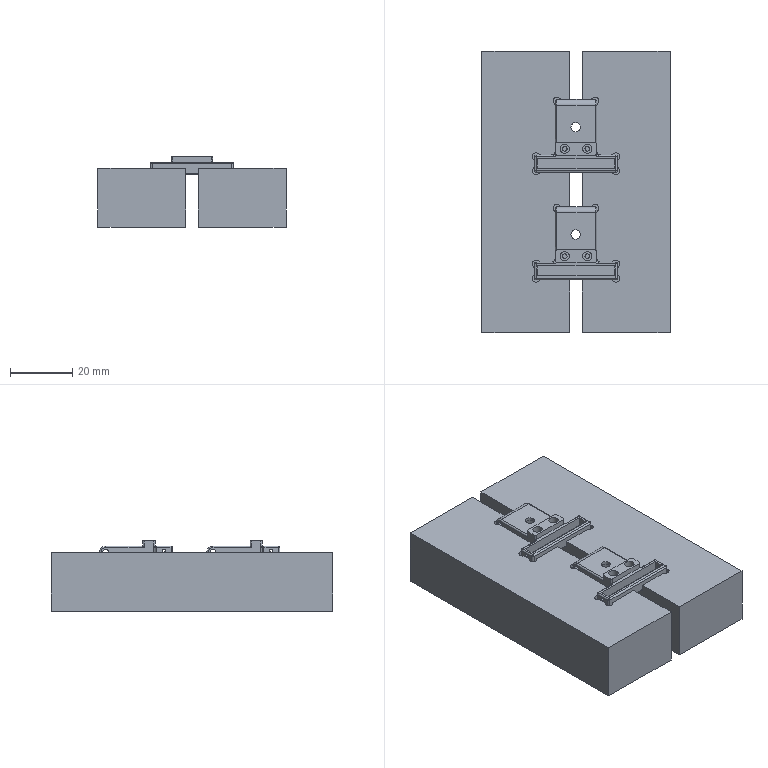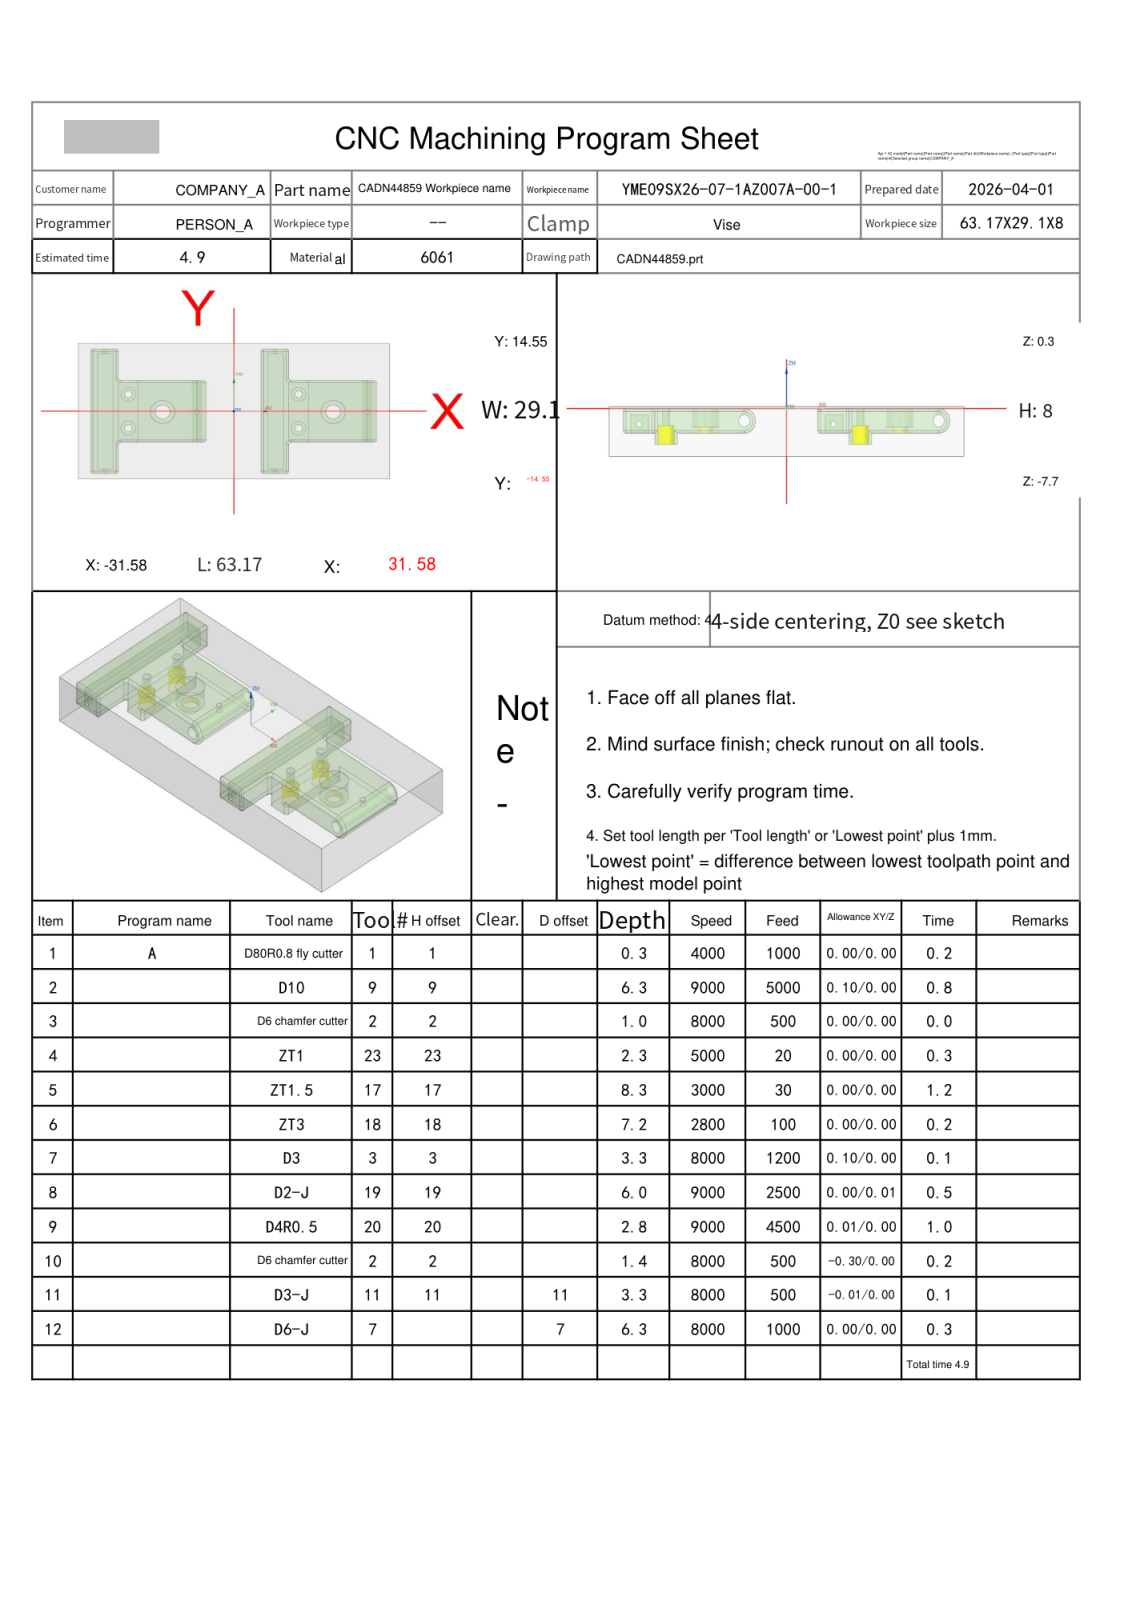NC program | NX | posted by the shop | part box 60.696 x 90.669 x 22.754 mm
Lines 1 to 833 of 3978:
%
O0001
(Machine time: 7.16 MIN)
(===Total Tool:11===)
(T1=D80R0.8 fly cutter D=80.  R=0.8  D-  H01 Z=0.    )
(T9=D10     D=10.  R=0.   D-  H09 Z=-5.95 )
(T2=D6 chamfer cutter   D=6.   R=0.   D-  H02 Z=-1.05 )
(T23=ZT1    D=1.   DR_a=118 D-  H23 Z=-2.   )
(T17=ZT1.5  D=1.5  DR_a=118 D-  H17 Z=-8.   )
(T18=ZT3    D=3.   DR_a=118 D-  H18 Z=-6.9  )
(T3=D3      D=3.   R=0.   D-  H03 Z=-3.   )
(T19=D2-J   D=2.   R=0.   D-  H19 Z=-5.7  )
(T20=D4R0.5 D=4.   R=0.5  D-  H20 Z=-2.5  )
(T11=D3-J   D=3.   R=0.   D11 H11 Z=-3.   )
(T7=D6-J    D=6.   R=0.   D7  H00 Z=-5.95 )
G80 G90 G17 G49 G40
G91 G28 Z0
M01
N1 T01 M06
(D80R0.8 fly cutter  D=80. R=0.8 H=01 ce=0.00 di=0.00)
G00 G90 G54 X-74.084 Y0.0 M03 S4000
G43 H01 Z20.
M08
Z2.
G01 Z0.0 F1000.
X-69.084
X69.084
X74.084
Z2.
G00 Z20.
G91 G28 Z0.0
M05
M09
G91 G28 Z0.0
M01
N2 T09 M06
(D10  D=10. R=0. H=09 ce=0.10 di=0.00)
G00 G90 G54 X.416 Y0.0 M03 S8000
G43 H09 Z20.
M08
Z.5
G01 Y12.848 Z.427 F5000.
G02 X6.016 Y18.448 Z.378 I5.6 J0.0
G01 X10.648 Z.352
G02 X16.248 Y12.848 Z.302 I0.0 J-5.6
G01 Y11.734 Z.296
X28.584 Z.226
G02 X34.184 Y6.134 Z.176 I0.0 J-5.6
G01 Y-6.134 Z.107
G02 X28.584 Y-11.734 Z.057 I-5.6 J0.0
G01 X16.248 Z-.013
Y-12.848 Z-.019
G02 X10.648 Y-18.448 Z-.069 I-5.6 J0.0
G01 X6.016 Z-.095
G02 X.416 Y-12.848 Z-.145 I0.0 J5.6
G01 Y12.848 Z-.29
G02 X6.016 Y18.448 Z-.339 I5.6 J0.0
G01 X10.648 Z-.366
G02 X16.248 Y12.848 Z-.415 I0.0 J-5.6
G01 Y11.734 Z-.422
X28.584 Z-.491
G02 X34.184 Y6.134 Z-.541 I0.0 J-5.6
G01 Y-6.134 Z-.61
G02 X28.584 Y-11.734 Z-.66 I-5.6 J0.0
G01 X16.248 Z-.73
Y-12.848 Z-.736
G02 X10.648 Y-18.448 Z-.786 I-5.6 J0.0
G01 X6.016 Z-.812
G02 X.416 Y-12.848 Z-.862 I0.0 J5.6
G01 Y12.848 Z-1.007
G02 X6.016 Y18.448 Z-1.057 I5.6 J0.0
G01 X10.648 Z-1.083
G02 X16.248 Y12.848 Z-1.132 I0.0 J-5.6
G01 Y11.734 Z-1.139
X28.584 Z-1.208
G02 X34.184 Y6.134 Z-1.258 I0.0 J-5.6
G01 Y-6.134 Z-1.327
G02 X28.584 Y-11.734 Z-1.377 I-5.6 J0.0
G01 X16.248 Z-1.447
Y-12.848 Z-1.453
G02 X10.648 Y-18.448 Z-1.503 I-5.6 J0.0
G01 X6.016 Z-1.529
G02 X.416 Y-12.848 Z-1.579 I0.0 J5.6
G01 Y12.848 Z-1.724
G02 X6.016 Y18.448 Z-1.774 I5.6 J0.0
G01 X10.648 Z-1.8
G02 X16.248 Y12.848 Z-1.85 I0.0 J-5.6
G01 Y11.734 Z-1.856
X28.584 Z-1.926
G02 X34.184 Y6.134 Z-1.975 I0.0 J-5.6
G01 Y-6.134 Z-2.045
G02 X28.584 Y-11.734 Z-2.094 I-5.6 J0.0
G01 X16.248 Z-2.164
Y-12.848 Z-2.17
G02 X10.648 Y-18.448 Z-2.22 I-5.6 J0.0
G01 X6.016 Z-2.246
G02 X.416 Y-12.848 Z-2.296 I0.0 J5.6
G01 Y12.848 Z-2.441
G02 X6.016 Y18.448 Z-2.491 I5.6 J0.0
G01 X10.648 Z-2.517
G02 X16.248 Y12.848 Z-2.567 I0.0 J-5.6
G01 Y11.734 Z-2.573
X28.584 Z-2.643
G02 X34.184 Y6.134 Z-2.692 I0.0 J-5.6
G01 Y-6.134 Z-2.762
G02 X28.584 Y-11.734 Z-2.811 I-5.6 J0.0
G01 X16.248 Z-2.881
Y-12.848 Z-2.887
G02 X10.648 Y-18.448 Z-2.937 I-5.6 J0.0
G01 X6.016 Z-2.963
G02 X.416 Y-12.848 Z-3.013 I0.0 J5.6
G01 Y12.848 Z-3.158
G02 X6.016 Y18.448 Z-3.208 I5.6 J0.0
G01 X10.648 Z-3.234
G02 X16.248 Y12.848 Z-3.284 I0.0 J-5.6
G01 Y11.734 Z-3.29
X28.584 Z-3.36
G02 X34.184 Y6.134 Z-3.409 I0.0 J-5.6
G01 Y-6.134 Z-3.479
G02 X28.584 Y-11.734 Z-3.528 I-5.6 J0.0
G01 X16.248 Z-3.598
Y-12.848 Z-3.605
G02 X10.648 Y-18.448 Z-3.654 I-5.6 J0.0
G01 X6.016 Z-3.68
G02 X.416 Y-12.848 Z-3.73 I0.0 J5.6
G01 Y12.848 Z-3.875
G02 X6.016 Y18.448 Z-3.925 I5.6 J0.0
G01 X10.648 Z-3.951
G02 X16.248 Y12.848 Z-4.001 I0.0 J-5.6
G01 Y11.734 Z-4.007
X28.584 Z-4.077
G02 X34.184 Y6.134 Z-4.127 I0.0 J-5.6
G01 Y-6.134 Z-4.196
G02 X28.584 Y-11.734 Z-4.246 I-5.6 J0.0
G01 X16.248 Z-4.315
Y-12.848 Z-4.322
G02 X10.648 Y-18.448 Z-4.371 I-5.6 J0.0
G01 X6.016 Z-4.397
G02 X.416 Y-12.848 Z-4.447 I0.0 J5.6
G01 Y12.848 Z-4.592
G02 X6.016 Y18.448 Z-4.642 I5.6 J0.0
G01 X10.648 Z-4.668
G02 X16.248 Y12.848 Z-4.718 I0.0 J-5.6
G01 Y11.734 Z-4.724
X28.584 Z-4.794
G02 X34.184 Y6.134 Z-4.844 I0.0 J-5.6
G01 Y-6.134 Z-4.913
G02 X28.584 Y-11.734 Z-4.963 I-5.6 J0.0
G01 X16.248 Z-5.032
Y-12.848 Z-5.039
G02 X10.648 Y-18.448 Z-5.088 I-5.6 J0.0
G01 X6.016 Z-5.115
G02 X.416 Y-12.848 Z-5.164 I0.0 J5.6
G01 Y12.848 Z-5.31
G02 X6.016 Y18.448 Z-5.359 I5.6 J0.0
G01 X10.648 Z-5.385
G02 X16.248 Y12.848 Z-5.435 I0.0 J-5.6
G01 Y11.734 Z-5.441
X28.584 Z-5.511
G02 X34.184 Y6.134 Z-5.561 I0.0 J-5.6
G01 Y-6.134 Z-5.63
G02 X28.584 Y-11.734 Z-5.68 I-5.6 J0.0
G01 X16.248 Z-5.75
Y-12.848 Z-5.756
G02 X10.648 Y-18.448 Z-5.806 I-5.6 J0.0
G01 X6.016 Z-5.832
G02 X.416 Y-12.848 Z-5.881 I0.0 J5.6
G01 Y0.0 Z-5.954
Y12.848
G02 X6.016 Y18.448 I5.6 J0.0
G01 X10.648
G02 X16.248 Y12.848 I0.0 J-5.6
G01 Y11.734
X28.584
G02 X34.184 Y6.134 I0.0 J-5.6
G01 Y-6.134
G02 X28.584 Y-11.734 I-5.6 J0.0
G01 X16.248
Y-12.848
G02 X10.648 Y-18.448 I-5.6 J0.0
G01 X6.016
G02 X.416 Y-12.848 I0.0 J5.6
G01 Y0.0
Y.5
Z-4.954
G00 Z20.
X-34.184 Y0.0
Z.5
G01 Y12.848 Z.427
G02 X-28.584 Y18.448 Z.378 I5.6 J0.0
G01 X-23.952 Z.352
G02 X-18.352 Y12.848 Z.302 I0.0 J-5.6
G01 Y11.734 Z.296
X-6.016 Z.226
G02 X-.416 Y6.134 Z.176 I0.0 J-5.6
G01 Y-6.134 Z.107
G02 X-6.016 Y-11.734 Z.057 I-5.6 J0.0
G01 X-18.352 Z-.013
Y-12.848 Z-.019
G02 X-23.952 Y-18.448 Z-.069 I-5.6 J0.0
G01 X-28.584 Z-.095
G02 X-34.184 Y-12.848 Z-.145 I0.0 J5.6
G01 Y12.848 Z-.29
G02 X-28.584 Y18.448 Z-.339 I5.6 J0.0
G01 X-23.952 Z-.366
G02 X-18.352 Y12.848 Z-.415 I0.0 J-5.6
G01 Y11.734 Z-.422
X-6.016 Z-.491
G02 X-.416 Y6.134 Z-.541 I0.0 J-5.6
G01 Y-6.134 Z-.61
G02 X-6.016 Y-11.734 Z-.66 I-5.6 J0.0
G01 X-18.352 Z-.73
Y-12.848 Z-.736
G02 X-23.952 Y-18.448 Z-.786 I-5.6 J0.0
G01 X-28.584 Z-.812
G02 X-34.184 Y-12.848 Z-.862 I0.0 J5.6
G01 Y12.848 Z-1.007
G02 X-28.584 Y18.448 Z-1.057 I5.6 J0.0
G01 X-23.952 Z-1.083
G02 X-18.352 Y12.848 Z-1.132 I0.0 J-5.6
G01 Y11.734 Z-1.139
X-6.016 Z-1.208
G02 X-.416 Y6.134 Z-1.258 I0.0 J-5.6
G01 Y-6.134 Z-1.327
G02 X-6.016 Y-11.734 Z-1.377 I-5.6 J0.0
G01 X-18.352 Z-1.447
Y-12.848 Z-1.453
G02 X-23.952 Y-18.448 Z-1.503 I-5.6 J0.0
G01 X-28.584 Z-1.529
G02 X-34.184 Y-12.848 Z-1.579 I0.0 J5.6
G01 Y12.848 Z-1.724
G02 X-28.584 Y18.448 Z-1.774 I5.6 J0.0
G01 X-23.952 Z-1.8
G02 X-18.352 Y12.848 Z-1.85 I0.0 J-5.6
G01 Y11.734 Z-1.856
X-6.016 Z-1.926
G02 X-.416 Y6.134 Z-1.975 I0.0 J-5.6
G01 Y-6.134 Z-2.045
G02 X-6.016 Y-11.734 Z-2.094 I-5.6 J0.0
G01 X-18.352 Z-2.164
Y-12.848 Z-2.17
G02 X-23.952 Y-18.448 Z-2.22 I-5.6 J0.0
G01 X-28.584 Z-2.246
G02 X-34.184 Y-12.848 Z-2.296 I0.0 J5.6
G01 Y12.848 Z-2.441
G02 X-28.584 Y18.448 Z-2.491 I5.6 J0.0
G01 X-23.952 Z-2.517
G02 X-18.352 Y12.848 Z-2.567 I0.0 J-5.6
G01 Y11.734 Z-2.573
X-6.016 Z-2.643
G02 X-.416 Y6.134 Z-2.692 I0.0 J-5.6
G01 Y-6.134 Z-2.762
G02 X-6.016 Y-11.734 Z-2.811 I-5.6 J0.0
G01 X-18.352 Z-2.881
Y-12.848 Z-2.887
G02 X-23.952 Y-18.448 Z-2.937 I-5.6 J0.0
G01 X-28.584 Z-2.963
G02 X-34.184 Y-12.848 Z-3.013 I0.0 J5.6
G01 Y12.848 Z-3.158
G02 X-28.584 Y18.448 Z-3.208 I5.6 J0.0
G01 X-23.952 Z-3.234
G02 X-18.352 Y12.848 Z-3.284 I0.0 J-5.6
G01 Y11.734 Z-3.29
X-6.016 Z-3.36
G02 X-.416 Y6.134 Z-3.409 I0.0 J-5.6
G01 Y-6.134 Z-3.479
G02 X-6.016 Y-11.734 Z-3.528 I-5.6 J0.0
G01 X-18.352 Z-3.598
Y-12.848 Z-3.605
G02 X-23.952 Y-18.448 Z-3.654 I-5.6 J0.0
G01 X-28.584 Z-3.68
G02 X-34.184 Y-12.848 Z-3.73 I0.0 J5.6
G01 Y12.848 Z-3.875
G02 X-28.584 Y18.448 Z-3.925 I5.6 J0.0
G01 X-23.952 Z-3.951
G02 X-18.352 Y12.848 Z-4.001 I0.0 J-5.6
G01 Y11.734 Z-4.007
X-6.016 Z-4.077
G02 X-.416 Y6.134 Z-4.127 I0.0 J-5.6
G01 Y-6.134 Z-4.196
G02 X-6.016 Y-11.734 Z-4.246 I-5.6 J0.0
G01 X-18.352 Z-4.315
Y-12.848 Z-4.322
G02 X-23.952 Y-18.448 Z-4.371 I-5.6 J0.0
G01 X-28.584 Z-4.397
G02 X-34.184 Y-12.848 Z-4.447 I0.0 J5.6
G01 Y12.848 Z-4.592
G02 X-28.584 Y18.448 Z-4.642 I5.6 J0.0
G01 X-23.952 Z-4.668
G02 X-18.352 Y12.848 Z-4.718 I0.0 J-5.6
G01 Y11.734 Z-4.724
X-6.016 Z-4.794
G02 X-.416 Y6.134 Z-4.844 I0.0 J-5.6
G01 Y-6.134 Z-4.913
G02 X-6.016 Y-11.734 Z-4.963 I-5.6 J0.0
G01 X-18.352 Z-5.032
Y-12.848 Z-5.039
G02 X-23.952 Y-18.448 Z-5.088 I-5.6 J0.0
G01 X-28.584 Z-5.115
G02 X-34.184 Y-12.848 Z-5.164 I0.0 J5.6
G01 Y12.848 Z-5.31
G02 X-28.584 Y18.448 Z-5.359 I5.6 J0.0
G01 X-23.952 Z-5.385
G02 X-18.352 Y12.848 Z-5.435 I0.0 J-5.6
G01 Y11.734 Z-5.441
X-6.016 Z-5.511
G02 X-.416 Y6.134 Z-5.561 I0.0 J-5.6
G01 Y-6.134 Z-5.63
G02 X-6.016 Y-11.734 Z-5.68 I-5.6 J0.0
G01 X-18.352 Z-5.75
Y-12.848 Z-5.756
G02 X-23.952 Y-18.448 Z-5.806 I-5.6 J0.0
G01 X-28.584 Z-5.832
G02 X-34.184 Y-12.848 Z-5.881 I0.0 J5.6
G01 Y0.0 Z-5.954
Y12.848
G02 X-28.584 Y18.448 I5.6 J0.0
G01 X-23.952
G02 X-18.352 Y12.848 I0.0 J-5.6
G01 Y11.734
X-6.016
G02 X-.416 Y6.134 I0.0 J-5.6
G01 Y-6.134
G02 X-6.016 Y-11.734 I-5.6 J0.0
G01 X-18.352
Y-12.848
G02 X-23.952 Y-18.448 I-5.6 J0.0
G01 X-28.584
G02 X-34.184 Y-12.848 I0.0 J5.6
G01 Y0.0
Y.5
Z-4.954
G00 Z20.
G00 G90 X-13.625 Y16.359 M03 S9000
Z10.3
Z.484
G01 Z-.016 F4500.
G03 X-8.625 Y11.359 I5. J0.0
G02 X-7.98 Y11.389 I.645 J-7.027
X-5.459 Y10.923 I0.0 J-7.056
X-2.164 Y6.134 I-1.832 J-4.788
G01 Y-6.134
G02 X-7.305 Y-11.341 I-5.311 J.102
G01 X-8.625 Y-11.359
X-8.627 Y-11.406 Z-.031
X-8.629 Y-11.438 Z-.045
X-7.544
X-7.305 Y-11.43
G03 X-2. Y-6.134 I-.154 J5.46
G01 Y6.134
G03 X-6.404 Y11.319 I-5.4 J-.123
X-8.1 Y11.451 I-1.696 J-10.865
X-8.629 Y11.438 I0.0 J-10.996
G01 Y11.489 Z-.07
Y11.525 Z-.095
G02 X-8.055 Y11.539 I.574 J-11.406
X-6.349 Y11.411 I0.0 J-11.42
X-1.812 Y6.134 I-.964 J-5.417
G01 Y-6.134
G02 X-5.053 Y-11.009 I-5.387 J.067
X-7.498 Y-11.521 I-2.445 J5.587
G01 X-7.544
X-8.614
X-8.629 Y-11.525
Y-11.606 Z-.166
X-8.614 Y-11.601
X-7.468 Y-11.6
G03 X-4.683 Y-10.963 I-.002 J6.41
X-1.618 Y-6.134 I-2.358 J4.883
G01 Y6.134
G03 X-2.579 Y9.173 I-5.492 J-.064
X-7.017 Y11.582 I-4.734 J-3.43
X-8.148 Y11.611 I-1.132 J-22.252
X-8.629 Y11.606 I0.0 J-22.281
G01 X-8.628 Y11.641 Z-.209
Y11.669 Z-.253
G02 X-8.102 Y11.675 I.526 J-20.023
X-6.855 Y11.637 I0.0 J-20.03
X-4.152 Y10.804 I-.457 J-6.288
X-1.442 Y6.134 I-2.751 J-4.718
G01 Y-6.134
G02 X-4.152 Y-10.804 I-5.458 J.046
X-6.855 Y-11.637 I-3.164 J5.47
X-8.102 Y-11.675 I-1.247 J19.991
X-8.628 Y-11.669 I0.0 J20.03
G01 Y-11.694 Z-.305
Y-11.713 Z-.357
G03 X-8.082 Y-11.719 I.546 J24.522
X-6.855 Y-11.688 I0.0 J24.528
X-4.223 Y-10.963 I-.357 J6.436
X-1.275 Y-6.134 I-2.571 J4.883
G01 Y6.134
G03 X-4.152 Y10.926 I-5.519 J-.054
X-6.855 Y11.688 I-3.06 J-5.674
X-8.082 Y11.719 I-1.227 J-24.486
X-8.628 Y11.713 I0.0 J-24.516
G01 X-8.621 Y11.733 Z-.479
G02 X-8.111 Y11.736 I.51 J-42.299
X-6.855 Y11.718 I0.0 J-42.302
X-3.702 Y10.775 I-.165 J-6.297
X-1.116 Y6.134 I-2.958 J-4.688
G01 Y-6.134
G02 X-4.023 Y-10.963 I-5.545 J.047
X-6.855 Y-11.718 I-3.002 J5.575
X-8.109 Y-11.737 I-1.255 J42.061
X-8.621 Y-11.733 I0.0 J42.08
G01 Z-.617
X-6.855
X-6.848
G03 X-3.702 Y-10.883 I0.0 J6.253
X-.971 Y-6.134 I-2.833 J4.789
G01 Y6.134
G03 X-3.845 Y10.963 I-5.558 J-.037
X-6.835 Y11.733 I-2.99 J-5.427
G01 X-6.855
X-8.621
Z-.768
G02 X-7.967 Y11.735 I.655 J-118.114
X-6.404 Y11.725 I0.0 J-118.116
X-2.497 Y10.068 I-.166 J-5.828
X-.84 Y6.134 I-3.906 J-3.961
G01 Y-6.134
G02 X-3.702 Y-10.975 I-5.581 J.033
X-6.404 Y-11.724 I-2.888 J5.174
X-7.99 Y-11.735 I-1.586 J113.299
X-8.621 Y-11.733 I0.0 J113.31
G01 Z-.932
X-6.404
G03 X-4.152 Y-11.264 I-.054 J5.912
X-.725 Y-6.134 I-2.169 J5.16
G01 Y6.134
G03 X-2.801 Y10.457 I-5.599 J-.029
X-6.404 Y11.733 I-3.645 J-4.57
G01 X-8.621
Z-1.106
X-6.404
X-6.323 Y11.734
G02 X-3.429 Y10.963 I0.0 J-5.821
X-.626 Y6.134 I-2.797 J-4.851
G01 Y-6.134
G02 X-5.954 Y-11.721 I-5.631 J.036
G01 X-6.404 Y-11.733
X-8.621
Z-1.29
X-6.404
X-5.954 Y-11.725
G03 X-.546 Y-6.134 I-.21 J5.614
G01 Y6.134
G03 X-5.954 Y11.723 I-5.612 J-.02
G01 X-6.404 Y11.733
X-8.621
Z-1.48
X-8.586
X-6.404
X-5.954 Y11.729
G02 X-.484 Y6.134 I-.141 J-5.609
G01 Y-6.134
G02 X-5.954 Y-11.73 I-5.612 J.015
G01 X-6.404 Y-11.733
X-8.621
Z-1.676
X-8.572
X-6.404
X-6.14
G03 X-5.053 Y-11.642 I-.013 J6.723
X-.442 Y-6.134 I-.997 J5.519
G01 Y6.134
G03 X-2.062 Y10.068 I-5.634 J-.019
X-5.954 Y11.733 I-4.012 J-4.
G01 X-6.404
X-8.586
X-8.621
Z-1.874
X-8.572
X-6.404
X-6.009
G02 X-.43 Y6.335 I-.012 J-5.595
G01 X-.423 Y6.144
X-.419 Y6.134
Y-6.134
G02 X-1.9 Y-9.921 I-5.662 J.031
X-5.954 Y-11.733 I-4.131 J3.801
G01 X-6.404
X-8.572
X-8.621
Y-11.734 Z-2.031
X-8.572 Y-11.733
X-6.404 Y-11.734
X-5.954 Y-11.733
G03 X-.417 Y-6.144 I-.063 J5.6
G01 X-.416 Y-6.041
Y6.144
G03 X-5.954 Y11.733 I-5.601 J-.012
G01 X-6.404 Y11.734
X-8.572 Y11.733
X-8.621 Y11.734
Z-2.187
X-5.954 Y11.733
G02 X-.416 Y6.144 I-.064 J-5.601
G01 Y-6.041
X-.417 Y-6.144
G02 X-5.954 Y-11.733 I-5.601 J.012
G01 X-8.621 Y-11.734
Z-2.344
X-8.572 Y-11.733
X-6.404 Y-11.734
X-5.954 Y-11.733
G03 X-.417 Y-6.144 I-.063 J5.601
G01 X-.416 Y-6.041
Y6.144
G03 X-5.954 Y11.733 I-5.601 J-.012
G01 X-6.404 Y11.734
X-8.572 Y11.733
X-8.621 Y11.734
Z-2.5
X-8.572 Y11.733
X-6.404 Y11.734
X-5.954 Y11.733
G02 X-.416 Y6.144 I-.064 J-5.601
G01 Y-6.041
X-.417 Y-6.144
G02 X-5.954 Y-11.733 I-5.601 J.012
G01 X-6.404 Y-11.734
X-8.572 Y-11.733
X-8.621 Y-11.734
G00 Z10.3
X20.973 Y16.359
Z.484
G01 Z-.016
G03 X25.973 Y11.359 I5. J0.0
G02 X26.589 Y11.384 I.616 J-7.534
X28.788 Y11.057 I0.0 J-7.559
X32.436 Y6.134 I-1.497 J-4.923
G01 Y-6.134
G02 X27.378 Y-11.338 I-5.304 J.095
G01 X26.928 Y-11.345
X26.027
X25.973 Y-11.359
X25.971 Y-11.406 Z-.031
X25.97 Y-11.438 Z-.045
X27.378 Y-11.427
G03 X32.6 Y-6.134 I-.192 J5.412
G01 Y6.134
G03 X28.279 Y11.308 I-5.361 J-.086
X26.516 Y11.452 I-1.763 J-10.726
X25.97 Y11.438 I0.0 J-10.87
G01 X25.971 Y11.489 Z-.07
Y11.525 Z-.095
G02 X26.578 Y11.544 I.607 J-9.58
X28.729 Y11.3 I0.0 J-9.599
X32.788 Y6.134 I-1.35 J-5.238
G01 Y-6.134
G02 X28.729 Y-11.3 I-5.408 J.072
X26.578 Y-11.544 I-2.152 J9.355
X25.971 Y-11.525 I0.0 J9.599
G01 Y-11.571 Z-.13
Y-11.606 Z-.166
G03 X26.533 Y-11.618 I.562 J12.687
X28.279 Y-11.498 I0.0 J12.699
X32.982 Y-6.134 I-.838 J5.478
G01 Y6.134
G03 X28.279 Y11.498 I-5.541 J-.115
X26.535 Y11.618 I-1.744 J-12.533
X25.971 Y11.606 I0.0 J-12.654
G01 Y11.641 Z-.209
Y11.669 Z-.253
G02 X26.55 Y11.68 I.579 J-14.155
X28.066 Y11.599 I0.0 J-14.167
X31.865 Y9.621 I-.629 J-5.844
X33.158 Y6.134 I-4.233 J-3.553
G01 Y-6.134
G02 X30.08 Y-11.005 I-5.481 J.055
X27.277 Y-11.661 I-2.842 J5.828
G01 X25.971 Y-11.669
Y-11.694 Z-.305
Y-11.713 Z-.357
G03 X26.541 Y-11.72 I.57 J22.855
X27.829 Y-11.684 I0.0 J22.862
X30.376 Y-10.963 I-.438 J6.411
X33.325 Y-6.134 I-2.568 J4.883
G01 Y6.134
G03 X30.376 Y10.963 I-5.518 J-.054
X27.829 Y11.682 I-2.977 J-5.677
X26.543 Y11.721 I-1.285 J-21.483
X25.971 Y11.713 I0.0 J-21.522
G01 X25.978 Y11.733 Z-.479
G02 X26.541 Y11.737 I.563 J-38.106
X27.829 Y11.715 I0.0 J-38.11
X30.58 Y10.963 I-.254 J-6.34
X33.484 Y6.134 I-2.644 J-4.878
G01 Y-6.134
G02 X30.531 Y-10.99 I-5.55 J.049
X27.829 Y-11.713 I-2.938 J5.568
X26.545 Y-11.738 I-1.284 J33.561
X25.978 Y-11.733 I0.0 J33.586
G01 Z-.617
X27.829 Y-11.73
G03 X30.531 Y-11.083 I-.056 J6.205
X33.629 Y-6.134 I-2.466 J4.988
G01 Y6.134
G03 X30.76 Y10.963 I-5.562 J-.038
X27.829 Y11.73 I-2.988 J-5.437
G01 X25.978 Y11.733
Z-.768
X27.829
X28.279 Y11.72
G02 X32.105 Y10.068 I-.249 J-5.834
X33.76 Y6.134 I-3.922 J-3.965
G01 Y-6.134
G02 X31.432 Y-10.636 I-5.576 J.03
G01 X31.147 Y-10.818
G02 X28.229 Y-11.721 I-3.097 J4.844
G01 X27.829 Y-11.733
X25.978
Z-.932
X27.829
X28.279 Y-11.731
G03 X30.982 Y-11.006 I-.122 J5.856
X33.875 Y-6.134 I-2.701 J4.9
G01 Y6.139
G03 X32.631 Y9.624 I-5.501 J0.0
X28.279 Y11.731 I-4.449 J-3.643
G01 X27.829 Y11.733
X25.978
Z-1.106
X28.279
X28.305
G02 X32.783 Y9.569 I0.0 J-5.717
X33.974 Y6.134 I-4.445 J-3.464
G01 Y-6.134
G02 X29.63 Y-11.575 I-5.613 J.026
X28.279 Y-11.733 I-1.383 J5.98
G01 X25.978
Z-1.29
X28.1
G03 X28.734 Y-11.717 I0.0 J12.332
X34.054 Y-6.134 I-.288 J5.601
G01 Y6.134
G03 X30.531 Y11.323 I-5.611 J-.019
X28.376 Y11.734 I-2.155 J-5.442
G01 X28.279 Y11.733
X25.978
Z-1.48
X26.027
X28.279
X28.729 Y11.724
G02 X34.116 Y6.134 I-.223 J-5.605
G01 Y-6.134
G02 X28.729 Y-11.724 I-5.608 J.014
G01 X28.279 Y-11.733
X25.978
Z-1.676
X28.552
G03 X29.229 Y-11.686 I0.0 J4.907
G01 X29.6 Y-11.635
X29.63 Y-11.622
G03 X34.158 Y-6.134 I-1.071 J5.495
G01 Y6.134
G03 X33.234 Y9.211 I-5.669 J-.026
X28.729 Y11.73 I-4.698 J-3.114
G01 X28.279 Y11.733
X25.978
Z-1.874
X28.279
X28.729 Y11.731
G02 X34.181 Y6.134 I-.168 J-5.617
G01 Y-6.134
G02 X28.729 Y-11.731 I-5.619 J.02
G01 X28.279 Y-11.733
X25.978
Y-11.734 Z-2.031
X28.279
X28.616 Y-11.731
G03 X34.185 Y-6.129 I-.034 J5.603
G01 Y6.129
G03 X28.616 Y11.731 I-5.603 J0.0
G01 X28.279 Y11.734
X25.978
Z-2.187
X28.279
X28.614 Y11.732
G02 X34.185 Y6.128 I-.032 J-5.603
G01 Y-6.129
G02 X28.614 Y-11.732 I-5.603 J0.0
G01 X28.279 Y-11.734
X25.978
Z-2.344
X28.279
X28.615 Y-11.732
G03 X34.185 Y-6.129 I-.033 J5.603
G01 Y6.128
G03 X28.615 Y11.732 I-5.603 J0.0
G01 X28.279 Y11.734
X25.978
Z-2.5
X28.279
X28.616 Y11.732
G02 X34.185 Y6.128 I-.034 J-5.603
G01 Y-6.129
G02 X28.616 Y-11.732 I-5.603 J0.0
G01 X28.279 Y-11.734
X25.978
G00 Z10.3
G91 G28 Z0.0
M05
M09
G91 G28 Z0.0
M01
N3 T02 M06
(D6 chamfer cutter  D=6. R=0. H=02 ce=0.00 di=0.00)
G00 G90 G54 X-21.452 Y3.634 M03 S8000
G43 H02 Z20.
M08
G98 G81 X-21.452 Y3.634 Z-.7 R1. F500.
Y-3.634
X-14.452 Y-.15
X13.148 Y3.634
Y-3.634
X20.148 Y-.15
X-7.516
X27.084
G80
G00 Z20.
G91 G28 Z0.0
M05
M09
G91 G28 Z0.0
M01
N4 T23 M06
(ZT1 D=1. DR_a=118 H=23)
G00 G90 G54 X-7.516 Y-.15 M03 S5000
G43 H23 Z20.
M08
G98 G83 X-7.516 Y-.15 Z-2. R1. F20. Q.8
X27.084
G80
G00 Z20.
G91 G28 Z0.0
M05
M09
G91 G28 Z0.0
M01
N5 T17 M06
(ZT1.5 D=1.5 DR_a=118 H=17)
G00 G90 G54 X-21.452 Y3.634 M03 S3000
G43 H17 Z20.
M08
G98 G83 X-21.452 Y3.634 Z-8. R1. F30. Q1.5
Y-3.634
X13.148
Y3.634
G80
G00 Z20.
G91 G28 Z0.0
M05
M09
G91 G28 Z0.0
M01
N6 T18 M06
(ZT3 D=3. DR_a=118 H=18)
G00 G90 G54 X-14.452 Y-.15 M03 S2800
G43 H18 Z20.
M08
G98 G83 X-14.452 Y-.15 Z-6.901 R1. F100. Q2.
X20.148
G80
G00 Z20.
G91 G28 Z0.0
M05
M09
G91 G28 Z0.0
M01
N7 T03 M06
(D3  D=3. R=0. H=03 ce=0.10 di=0.00)
G00 G90 G54 X-14.452 Y-.15 M03 S8000
G43 H03 Z20.
M08
Z.5
G03 X-14.002 Y.3 I0.0 J.45 F1200.
X-14.452 Y.75 I-.45 J0.0
X-14.452 Y.75 Z.2 I0.0 J-.9
X-14.452 Y.75 Z-.1 I0.0 J-.9
X-14.452 Y.75 Z-.4 I0.0 J-.9
X-14.452 Y.75 Z-.7 I0.0 J-.9
X-14.452 Y.75 Z-1. I0.0 J-.9
X-14.452 Y.75 Z-1.3 I0.0 J-.9
X-14.452 Y.75 Z-1.6 I0.0 J-.9
X-14.452 Y.75 Z-1.9 I0.0 J-.9
X-14.452 Y.75 Z-2.2 I0.0 J-.9
X-14.452 Y.75 Z-2.5 I0.0 J-.9
X-14.452 Y.75 Z-2.8 I0.0 J-.9
X-13.673 Y-.6 Z-3. I0.0 J-.9
X-13.552 Y-.15 I-.779 J.45
X-14.452 Y.75 I-.9 J0.0
X-15.352 Y-.15 I0.0 J-.9
X-14.452 Y-1.05 I.9 J0.0
X-13.673 Y-.6 I0.0 J.9
X-13.613 Y-.375 I-.39 J.225
X-14.063 Y.075 I-.45 J0.0
X-14.452 Y-.15 I0.0 J-.45
G00 Z20.
X20.148
Z.5
G03 X20.598 Y.3 I0.0 J.45
X20.148 Y.75 I-.45 J0.0
X20.148 Y.75 Z.2 I0.0 J-.9
X20.148 Y.75 Z-.1 I0.0 J-.9
X20.148 Y.75 Z-.4 I0.0 J-.9
X20.148 Y.75 Z-.7 I0.0 J-.9
X20.148 Y.75 Z-1. I0.0 J-.9
X20.148 Y.75 Z-1.3 I0.0 J-.9
X20.148 Y.75 Z-1.6 I0.0 J-.9
X20.148 Y.75 Z-1.9 I0.0 J-.9
X20.148 Y.75 Z-2.2 I0.0 J-.9
X20.148 Y.75 Z-2.5 I0.0 J-.9
X20.148 Y.75 Z-2.8 I0.0 J-.9
X20.927 Y-.6 Z-3. I0.0 J-.9
X21.048 Y-.15 I-.779 J.45
X20.148 Y.75 I-.9 J0.0
X19.248 Y-.15 I0.0 J-.9
X20.148 Y-1.05 I.9 J0.0
X20.927 Y-.6 I0.0 J.9
X20.987 Y-.375 I-.39 J.225
X20.537 Y.075 I-.45 J0.0
X20.148 Y-.15 I0.0 J-.45
G00 Z20.
G91 G28 Z0.0
M05
M09
G91 G28 Z0.0
M01